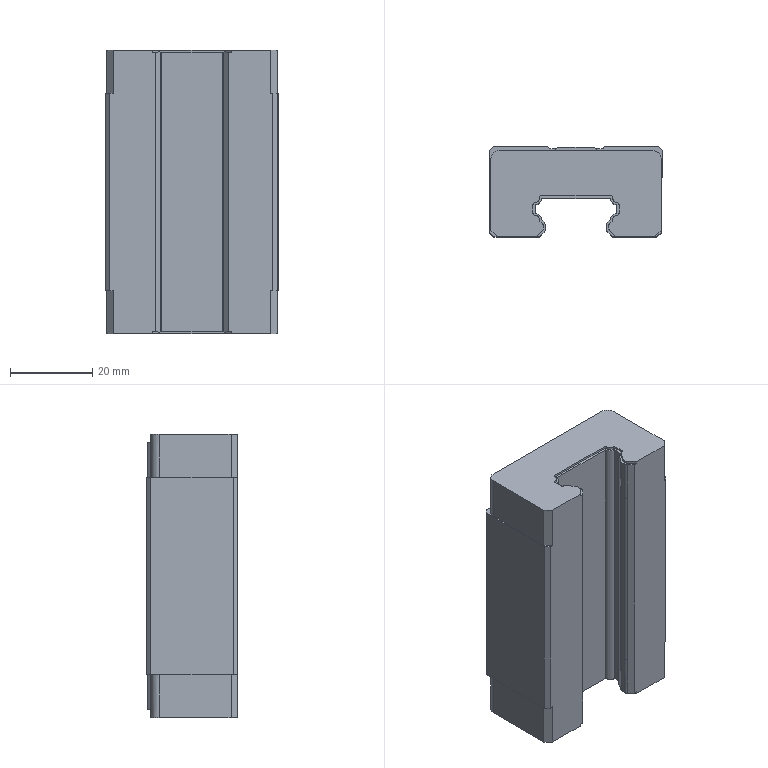Part | NX | features BREP 2 | 1 solid | 167 faces | box 42 x 22 x 69.1 mm | volume 50239 mm3 | plane 83 | cylinder 72 | cone 12 | commonest cylinder face diameters 1.6 x16 2.5 x12 1 x8 5 x8 0.457 x4 0.461 x4